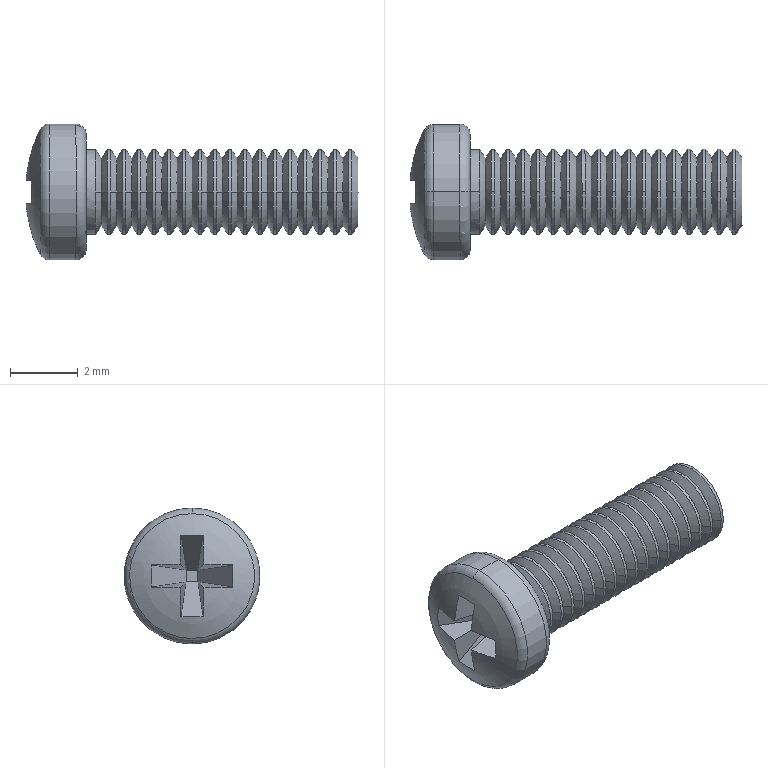Part | SolidWorks | features BaseBody 1 | 1 solid | 128 faces | box 9.771 x 4.001 x 4 mm | volume 50.579 mm3 | cone 70 | cylinder 38 | plane 15 | torus 4 | sphere 1 | commonest cylinder face diameters 2.5 x36 4 x2